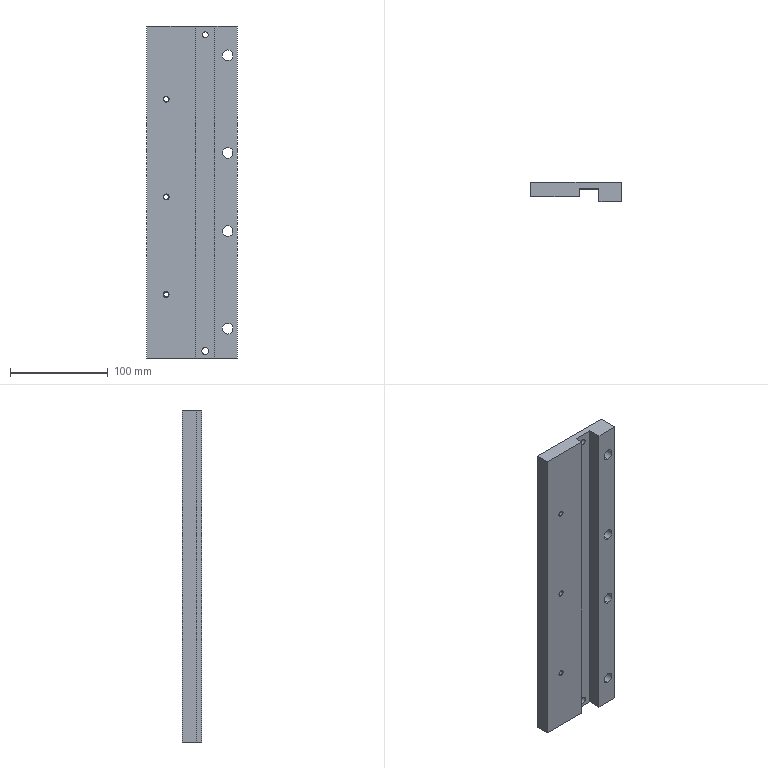Part | STEP file | 1 solid | 54 faces | box 92.98 x 19.5 x 340 mm | volume 429888 mm3 | cylinder 26 | cone 14 | plane 14 | commonest cylinder face diameters 11 x8 18 x8 5 x6 5.96 x2 7 x2